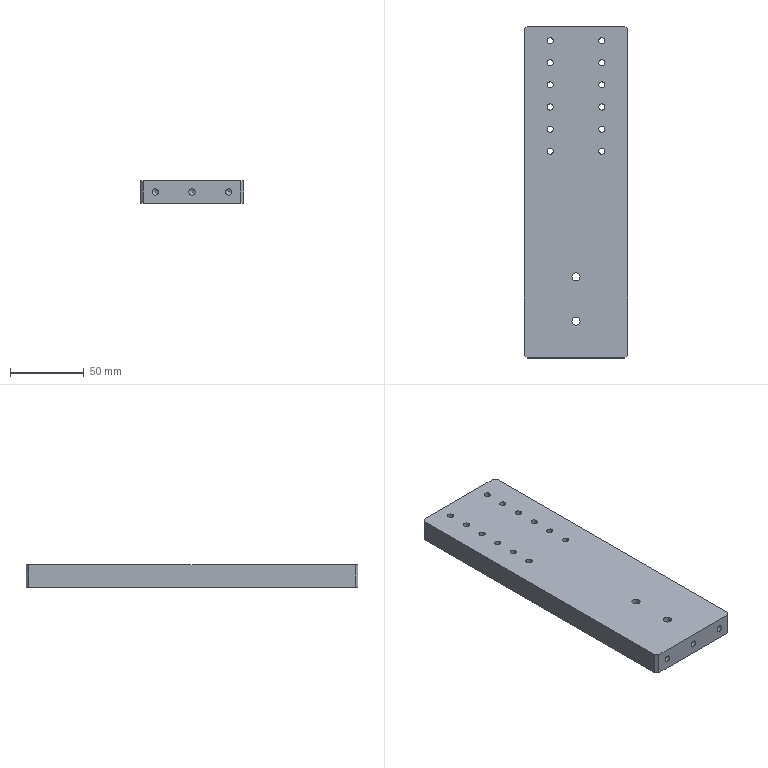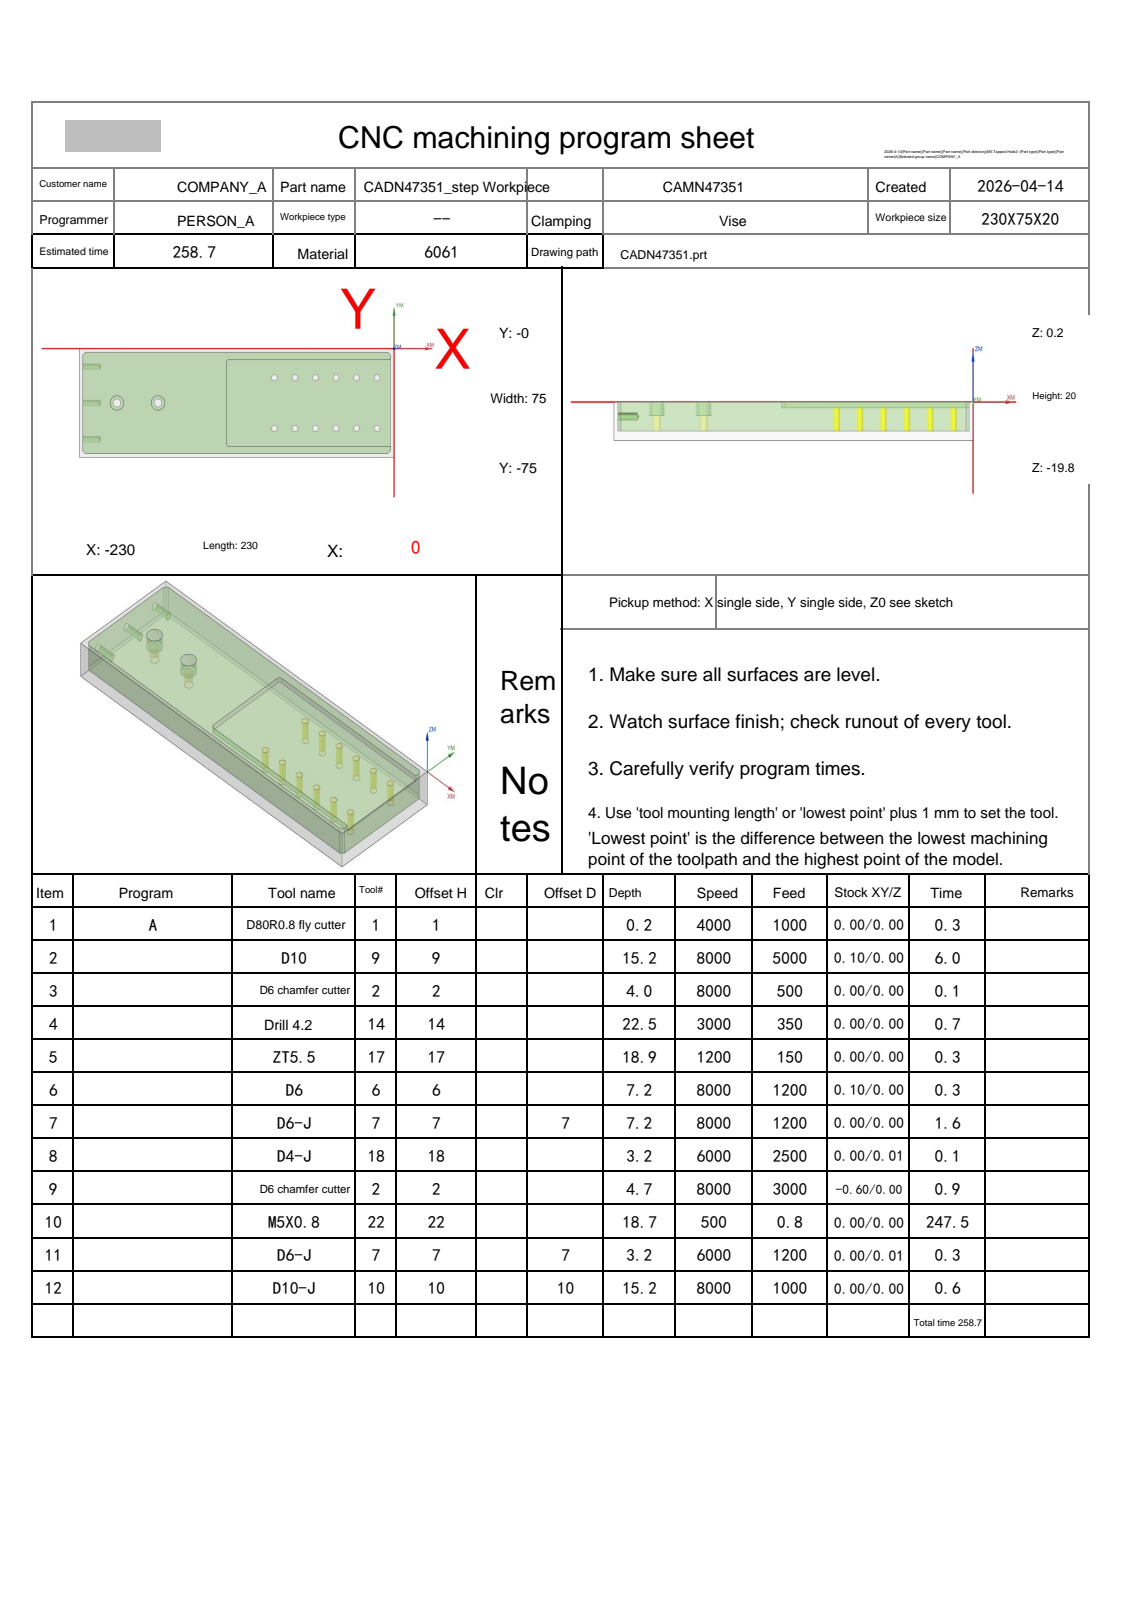NC program | NX | posted by the shop | part box 70 x 225 x 15 mm
Whole program, first 1531 of 2028 lines:
%
O0001
(Machine time: 493.75 MIN)
(===Total Tool:10===)
(T1=D80R0.8 fly cutter D=80.  R=0.8  D-  H01 Z=0.    )
(T9=D10     D=10.  R=0.   D-  H09 Z=-15.2 )
(T2=D6 chamfer cutter   D=6.   R=0.   D-  H02 Z=-4.5  )
(T14=Drill 4.2  D=4.2  DR_a=118 D-  H14 Z=-22.26)
(T17=ZT5.5  D=5.5  DR_a=118 D-  H17 Z=-18.65)
(T6=D6      D=6.   R=0.   D-  H06 Z=-7.   )
(T7=D6-J    D=6.   R=0.   D7  H07 Z=-7.   )
(T18=D4-J   D=4.   R=0.   D-  H18 Z=-3.   )
(T22=M5X0.8 D=4.2  DR_a=180 D-  H22 Z=-18.5 )
(T10=D10-J  D=10.  R=0.   D10 H10 Z=-15.2 )
G80 G90 G17 G49 G40
G91 G28 Z0
M01
N1 T01 M06
(D80R0.8 fly cutter  D=80. R=0.8 H=01 ce=0.00 di=0.00)
G00 G90 G54 X-272.5 Y-37.5 M03 S4000
G43 H01 Z20.
M08
Z2.
G01 Z0.0 F1000.
X-267.5
X37.5
X42.5
Z2.
G00 Z20.
G91 G28 Z0.0
M05
M09
G91 G28 Z0.0
M01
N2 T09 M06
(D10  D=10. R=0. H=09 ce=0.10 di=0.00)
G00 G90 G54 X-115. Y2.6 M03 S8000
G43 H09 Z20.
M08
Z.5
G01 X-4.5 Z.412 F5000.
G02 X-.894 Y1.106 Z.409 I0.0 J-5.1
G01 X1.106 Y-.894 Z.407
G02 X2.6 Y-4.5 Z.404 I-3.606 J-3.606
G01 Y-70.5 Z.351
G02 X1.106 Y-74.106 Z.348 I-5.1 J0.0
G01 X-.894 Y-76.106 Z.346
G02 X-4.5 Y-77.6 Z.343 I-3.606 J3.606
G01 X-225.5 Z.167
G02 X-229.106 Y-76.106 Z.164 I0.0 J5.1
G01 X-231.106 Y-74.106 Z.161
G02 X-232.6 Y-70.5 Z.158 I3.606 J3.606
G01 Y-4.5 Z.106
G02 X-231.106 Y-.894 Z.103 I5.1 J0.0
G01 X-229.106 Y1.106 Z.1
G02 X-225.5 Y2.6 Z.097 I3.606 J-3.606
G01 X-4.5 Z-.078
G02 X-.894 Y1.106 Z-.082 I0.0 J-5.1
G01 X1.106 Y-.894 Z-.084
G02 X2.6 Y-4.5 Z-.087 I-3.606 J-3.606
G01 Y-70.5 Z-.14
G02 X1.106 Y-74.106 Z-.143 I-5.1 J0.0
G01 X-.894 Y-76.106 Z-.145
G02 X-4.5 Y-77.6 Z-.148 I-3.606 J3.606
G01 X-225.5 Z-.324
G02 X-229.106 Y-76.106 Z-.327 I0.0 J5.1
G01 X-231.106 Y-74.106 Z-.329
G02 X-232.6 Y-70.5 Z-.332 I3.606 J3.606
G01 Y-4.5 Z-.385
G02 X-231.106 Y-.894 Z-.388 I5.1 J0.0
G01 X-229.106 Y1.106 Z-.39
G02 X-225.5 Y2.6 Z-.393 I3.606 J-3.606
G01 X-4.5 Z-.569
G02 X-.894 Y1.106 Z-.572 I0.0 J-5.1
G01 X1.106 Y-.894 Z-.574
G02 X2.6 Y-4.5 Z-.578 I-3.606 J-3.606
G01 Y-70.5 Z-.63
G02 X1.106 Y-74.106 Z-.633 I-5.1 J0.0
G01 X-.894 Y-76.106 Z-.636
G02 X-4.5 Y-77.6 Z-.639 I-3.606 J3.606
G01 X-225.5 Z-.814
G02 X-229.106 Y-76.106 Z-.818 I0.0 J5.1
G01 X-231.106 Y-74.106 Z-.82
G02 X-232.6 Y-70.5 Z-.823 I3.606 J3.606
G01 Y-4.5 Z-.875
G02 X-231.106 Y-.894 Z-.879 I5.1 J0.0
G01 X-229.106 Y1.106 Z-.881
G02 X-225.5 Y2.6 Z-.884 I3.606 J-3.606
G01 X-4.5 Z-1.06
G02 X-.894 Y1.106 Z-1.063 I0.0 J-5.1
G01 X1.106 Y-.894 Z-1.065
G02 X2.6 Y-4.5 Z-1.068 I-3.606 J-3.606
G01 Y-70.5 Z-1.121
G02 X1.106 Y-74.106 Z-1.124 I-5.1 J0.0
G01 X-.894 Y-76.106 Z-1.126
G02 X-4.5 Y-77.6 Z-1.129 I-3.606 J3.606
G01 X-225.5 Z-1.305
G02 X-229.106 Y-76.106 Z-1.308 I0.0 J5.1
G01 X-231.106 Y-74.106 Z-1.31
G02 X-232.6 Y-70.5 Z-1.314 I3.606 J3.606
G01 Y-4.5 Z-1.366
G02 X-231.106 Y-.894 Z-1.369 I5.1 J0.0
G01 X-229.106 Y1.106 Z-1.372
G02 X-225.5 Y2.6 Z-1.375 I3.606 J-3.606
G01 X-4.5 Z-1.55
G02 X-.894 Y1.106 Z-1.554 I0.0 J-5.1
G01 X1.106 Y-.894 Z-1.556
G02 X2.6 Y-4.5 Z-1.559 I-3.606 J-3.606
G01 Y-70.5 Z-1.611
G02 X1.106 Y-74.106 Z-1.615 I-5.1 J0.0
G01 X-.894 Y-76.106 Z-1.617
G02 X-4.5 Y-77.6 Z-1.62 I-3.606 J3.606
G01 X-225.5 Z-1.796
G02 X-229.106 Y-76.106 Z-1.799 I0.0 J5.1
G01 X-231.106 Y-74.106 Z-1.801
G02 X-232.6 Y-70.5 Z-1.804 I3.606 J3.606
G01 Y-4.5 Z-1.857
G02 X-231.106 Y-.894 Z-1.86 I5.1 J0.0
G01 X-229.106 Y1.106 Z-1.862
G02 X-225.5 Y2.6 Z-1.865 I3.606 J-3.606
G01 X-4.5 Z-2.041
G02 X-.894 Y1.106 Z-2.044 I0.0 J-5.1
G01 X1.106 Y-.894 Z-2.046
G02 X2.6 Y-4.5 Z-2.05 I-3.606 J-3.606
G01 Y-70.5 Z-2.102
G02 X1.106 Y-74.106 Z-2.105 I-5.1 J0.0
G01 X-.894 Y-76.106 Z-2.107
G02 X-4.5 Y-77.6 Z-2.111 I-3.606 J3.606
G01 X-225.5 Z-2.286
G02 X-229.106 Y-76.106 Z-2.289 I0.0 J5.1
G01 X-231.106 Y-74.106 Z-2.292
G02 X-232.6 Y-70.5 Z-2.295 I3.606 J3.606
G01 Y-4.5 Z-2.347
G02 X-231.106 Y-.894 Z-2.351 I5.1 J0.0
G01 X-229.106 Y1.106 Z-2.353
G02 X-225.5 Y2.6 Z-2.356 I3.606 J-3.606
G01 X-4.5 Z-2.532
G02 X-.894 Y1.106 Z-2.535 I0.0 J-5.1
G01 X1.106 Y-.894 Z-2.537
G02 X2.6 Y-4.5 Z-2.54 I-3.606 J-3.606
G01 Y-70.5 Z-2.593
G02 X1.106 Y-74.106 Z-2.596 I-5.1 J0.0
G01 X-.894 Y-76.106 Z-2.598
G02 X-4.5 Y-77.6 Z-2.601 I-3.606 J3.606
G01 X-225.5 Z-2.777
G02 X-229.106 Y-76.106 Z-2.78 I0.0 J5.1
G01 X-231.106 Y-74.106 Z-2.782
G02 X-232.6 Y-70.5 Z-2.785 I3.606 J3.606
G01 Y-4.5 Z-2.838
G02 X-231.106 Y-.894 Z-2.841 I5.1 J0.0
G01 X-229.106 Y1.106 Z-2.843
G02 X-225.5 Y2.6 Z-2.847 I3.606 J-3.606
G01 X-4.5 Z-3.022
G02 X-.894 Y1.106 Z-3.025 I0.0 J-5.1
G01 X1.106 Y-.894 Z-3.028
G02 X2.6 Y-4.5 Z-3.031 I-3.606 J-3.606
G01 Y-70.5 Z-3.083
G02 X1.106 Y-74.106 Z-3.086 I-5.1 J0.0
G01 X-.894 Y-76.106 Z-3.089
G02 X-4.5 Y-77.6 Z-3.092 I-3.606 J3.606
G01 X-225.5 Z-3.268
G02 X-229.106 Y-76.106 Z-3.271 I0.0 J5.1
G01 X-231.106 Y-74.106 Z-3.273
G02 X-232.6 Y-70.5 Z-3.276 I3.606 J3.606
G01 Y-4.5 Z-3.329
G02 X-231.106 Y-.894 Z-3.332 I5.1 J0.0
G01 X-229.106 Y1.106 Z-3.334
G02 X-225.5 Y2.6 Z-3.337 I3.606 J-3.606
G01 X-4.5 Z-3.513
G02 X-.894 Y1.106 Z-3.516 I0.0 J-5.1
G01 X1.106 Y-.894 Z-3.518
G02 X2.6 Y-4.5 Z-3.521 I-3.606 J-3.606
G01 Y-70.5 Z-3.574
G02 X1.106 Y-74.106 Z-3.577 I-5.1 J0.0
G01 X-.894 Y-76.106 Z-3.579
G02 X-4.5 Y-77.6 Z-3.582 I-3.606 J3.606
G01 X-225.5 Z-3.758
G02 X-229.106 Y-76.106 Z-3.761 I0.0 J5.1
G01 X-231.106 Y-74.106 Z-3.764
G02 X-232.6 Y-70.5 Z-3.767 I3.606 J3.606
G01 Y-4.5 Z-3.819
G02 X-231.106 Y-.894 Z-3.822 I5.1 J0.0
G01 X-229.106 Y1.106 Z-3.825
G02 X-225.5 Y2.6 Z-3.828 I3.606 J-3.606
G01 X-4.5 Z-4.003
G02 X-.894 Y1.106 Z-4.007 I0.0 J-5.1
G01 X1.106 Y-.894 Z-4.009
G02 X2.6 Y-4.5 Z-4.012 I-3.606 J-3.606
G01 Y-70.5 Z-4.065
G02 X1.106 Y-74.106 Z-4.068 I-5.1 J0.0
G01 X-.894 Y-76.106 Z-4.07
G02 X-4.5 Y-77.6 Z-4.073 I-3.606 J3.606
G01 X-225.5 Z-4.249
G02 X-229.106 Y-76.106 Z-4.252 I0.0 J5.1
G01 X-231.106 Y-74.106 Z-4.254
G02 X-232.6 Y-70.5 Z-4.257 I3.606 J3.606
G01 Y-4.5 Z-4.31
G02 X-231.106 Y-.894 Z-4.313 I5.1 J0.0
G01 X-229.106 Y1.106 Z-4.315
G02 X-225.5 Y2.6 Z-4.318 I3.606 J-3.606
G01 X-4.5 Z-4.494
G02 X-.894 Y1.106 Z-4.497 I0.0 J-5.1
G01 X1.106 Y-.894 Z-4.499
G02 X2.6 Y-4.5 Z-4.503 I-3.606 J-3.606
G01 Y-70.5 Z-4.555
G02 X1.106 Y-74.106 Z-4.558 I-5.1 J0.0
G01 X-.894 Y-76.106 Z-4.561
G02 X-4.5 Y-77.6 Z-4.564 I-3.606 J3.606
G01 X-225.5 Z-4.739
G02 X-229.106 Y-76.106 Z-4.743 I0.0 J5.1
G01 X-231.106 Y-74.106 Z-4.745
G02 X-232.6 Y-70.5 Z-4.748 I3.606 J3.606
G01 Y-4.5 Z-4.8
G02 X-231.106 Y-.894 Z-4.804 I5.1 J0.0
G01 X-229.106 Y1.106 Z-4.806
G02 X-225.5 Y2.6 Z-4.809 I3.606 J-3.606
G01 X-4.5 Z-4.985
G02 X-.894 Y1.106 Z-4.988 I0.0 J-5.1
G01 X1.106 Y-.894 Z-4.99
G02 X2.6 Y-4.5 Z-4.993 I-3.606 J-3.606
G01 Y-70.5 Z-5.046
G02 X1.106 Y-74.106 Z-5.049 I-5.1 J0.0
G01 X-.894 Y-76.106 Z-5.051
G02 X-4.5 Y-77.6 Z-5.054 I-3.606 J3.606
G01 X-225.5 Z-5.23
G02 X-229.106 Y-76.106 Z-5.233 I0.0 J5.1
G01 X-231.106 Y-74.106 Z-5.235
G02 X-232.6 Y-70.5 Z-5.239 I3.606 J3.606
G01 Y-4.5 Z-5.291
G02 X-231.106 Y-.894 Z-5.294 I5.1 J0.0
G01 X-229.106 Y1.106 Z-5.297
G02 X-225.5 Y2.6 Z-5.3 I3.606 J-3.606
G01 X-4.5 Z-5.475
G02 X-.894 Y1.106 Z-5.479 I0.0 J-5.1
G01 X1.106 Y-.894 Z-5.481
G02 X2.6 Y-4.5 Z-5.484 I-3.606 J-3.606
G01 Y-70.5 Z-5.536
G02 X1.106 Y-74.106 Z-5.54 I-5.1 J0.0
G01 X-.894 Y-76.106 Z-5.542
G02 X-4.5 Y-77.6 Z-5.545 I-3.606 J3.606
G01 X-225.5 Z-5.721
G02 X-229.106 Y-76.106 Z-5.724 I0.0 J5.1
G01 X-231.106 Y-74.106 Z-5.726
G02 X-232.6 Y-70.5 Z-5.729 I3.606 J3.606
G01 Y-4.5 Z-5.782
G02 X-231.106 Y-.894 Z-5.785 I5.1 J0.0
G01 X-229.106 Y1.106 Z-5.787
G02 X-225.5 Y2.6 Z-5.79 I3.606 J-3.606
G01 X-4.5 Z-5.966
G02 X-.894 Y1.106 Z-5.969 I0.0 J-5.1
G01 X1.106 Y-.894 Z-5.971
G02 X2.6 Y-4.5 Z-5.975 I-3.606 J-3.606
G01 Y-70.5 Z-6.027
G02 X1.106 Y-74.106 Z-6.03 I-5.1 J0.0
G01 X-.894 Y-76.106 Z-6.032
G02 X-4.5 Y-77.6 Z-6.036 I-3.606 J3.606
G01 X-225.5 Z-6.211
G02 X-229.106 Y-76.106 Z-6.214 I0.0 J5.1
G01 X-231.106 Y-74.106 Z-6.217
G02 X-232.6 Y-70.5 Z-6.22 I3.606 J3.606
G01 Y-4.5 Z-6.272
G02 X-231.106 Y-.894 Z-6.276 I5.1 J0.0
G01 X-229.106 Y1.106 Z-6.278
G02 X-225.5 Y2.6 Z-6.281 I3.606 J-3.606
G01 X-4.5 Z-6.457
G02 X-.894 Y1.106 Z-6.46 I0.0 J-5.1
G01 X1.106 Y-.894 Z-6.462
G02 X2.6 Y-4.5 Z-6.465 I-3.606 J-3.606
G01 Y-70.5 Z-6.518
G02 X1.106 Y-74.106 Z-6.521 I-5.1 J0.0
G01 X-.894 Y-76.106 Z-6.523
G02 X-4.5 Y-77.6 Z-6.526 I-3.606 J3.606
G01 X-225.5 Z-6.702
G02 X-229.106 Y-76.106 Z-6.705 I0.0 J5.1
G01 X-231.106 Y-74.106 Z-6.707
G02 X-232.6 Y-70.5 Z-6.71 I3.606 J3.606
G01 Y-4.5 Z-6.763
G02 X-231.106 Y-.894 Z-6.766 I5.1 J0.0
G01 X-229.106 Y1.106 Z-6.768
G02 X-225.5 Y2.6 Z-6.772 I3.606 J-3.606
G01 X-4.5 Z-6.947
G02 X-.894 Y1.106 Z-6.95 I0.0 J-5.1
G01 X1.106 Y-.894 Z-6.953
G02 X2.6 Y-4.5 Z-6.956 I-3.606 J-3.606
G01 Y-70.5 Z-7.008
G02 X1.106 Y-74.106 Z-7.011 I-5.1 J0.0
G01 X-.894 Y-76.106 Z-7.014
G02 X-4.5 Y-77.6 Z-7.017 I-3.606 J3.606
G01 X-225.5 Z-7.193
G02 X-229.106 Y-76.106 Z-7.196 I0.0 J5.1
G01 X-231.106 Y-74.106 Z-7.198
G02 X-232.6 Y-70.5 Z-7.201 I3.606 J3.606
G01 Y-4.5 Z-7.254
G02 X-231.106 Y-.894 Z-7.257 I5.1 J0.0
G01 X-229.106 Y1.106 Z-7.259
G02 X-225.5 Y2.6 Z-7.262 I3.606 J-3.606
G01 X-4.5 Z-7.438
G02 X-.894 Y1.106 Z-7.441 I0.0 J-5.1
G01 X1.106 Y-.894 Z-7.443
G02 X2.6 Y-4.5 Z-7.446 I-3.606 J-3.606
G01 Y-70.5 Z-7.499
G02 X1.106 Y-74.106 Z-7.502 I-5.1 J0.0
G01 X-.894 Y-76.106 Z-7.504
G02 X-4.5 Y-77.6 Z-7.507 I-3.606 J3.606
G01 X-225.5 Z-7.683
G02 X-229.106 Y-76.106 Z-7.686 I0.0 J5.1
G01 X-231.106 Y-74.106 Z-7.689
G02 X-232.6 Y-70.5 Z-7.692 I3.606 J3.606
G01 Y-4.5 Z-7.744
G02 X-231.106 Y-.894 Z-7.747 I5.1 J0.0
G01 X-229.106 Y1.106 Z-7.75
G02 X-225.5 Y2.6 Z-7.753 I3.606 J-3.606
G01 X-4.5 Z-7.928
G02 X-.894 Y1.106 Z-7.932 I0.0 J-5.1
G01 X1.106 Y-.894 Z-7.934
G02 X2.6 Y-4.5 Z-7.937 I-3.606 J-3.606
G01 Y-70.5 Z-7.99
G02 X1.106 Y-74.106 Z-7.993 I-5.1 J0.0
G01 X-.894 Y-76.106 Z-7.995
G02 X-4.5 Y-77.6 Z-7.998 I-3.606 J3.606
G01 X-225.5 Z-8.174
G02 X-229.106 Y-76.106 Z-8.177 I0.0 J5.1
G01 X-231.106 Y-74.106 Z-8.179
G02 X-232.6 Y-70.5 Z-8.182 I3.606 J3.606
G01 Y-4.5 Z-8.235
G02 X-231.106 Y-.894 Z-8.238 I5.1 J0.0
G01 X-229.106 Y1.106 Z-8.24
G02 X-225.5 Y2.6 Z-8.243 I3.606 J-3.606
G01 X-4.5 Z-8.419
G02 X-.894 Y1.106 Z-8.422 I0.0 J-5.1
G01 X1.106 Y-.894 Z-8.424
G02 X2.6 Y-4.5 Z-8.428 I-3.606 J-3.606
G01 Y-70.5 Z-8.48
G02 X1.106 Y-74.106 Z-8.483 I-5.1 J0.0
G01 X-.894 Y-76.106 Z-8.486
G02 X-4.5 Y-77.6 Z-8.489 I-3.606 J3.606
G01 X-225.5 Z-8.664
G02 X-229.106 Y-76.106 Z-8.668 I0.0 J5.1
G01 X-231.106 Y-74.106 Z-8.67
G02 X-232.6 Y-70.5 Z-8.673 I3.606 J3.606
G01 Y-4.5 Z-8.725
G02 X-231.106 Y-.894 Z-8.729 I5.1 J0.0
G01 X-229.106 Y1.106 Z-8.731
G02 X-225.5 Y2.6 Z-8.734 I3.606 J-3.606
G01 X-4.5 Z-8.91
G02 X-.894 Y1.106 Z-8.913 I0.0 J-5.1
G01 X1.106 Y-.894 Z-8.915
G02 X2.6 Y-4.5 Z-8.918 I-3.606 J-3.606
G01 Y-70.5 Z-8.971
G02 X1.106 Y-74.106 Z-8.974 I-5.1 J0.0
G01 X-.894 Y-76.106 Z-8.976
G02 X-4.5 Y-77.6 Z-8.979 I-3.606 J3.606
G01 X-225.5 Z-9.155
G02 X-229.106 Y-76.106 Z-9.158 I0.0 J5.1
G01 X-231.106 Y-74.106 Z-9.16
G02 X-232.6 Y-70.5 Z-9.164 I3.606 J3.606
G01 Y-4.5 Z-9.216
G02 X-231.106 Y-.894 Z-9.219 I5.1 J0.0
G01 X-229.106 Y1.106 Z-9.222
G02 X-225.5 Y2.6 Z-9.225 I3.606 J-3.606
G01 X-4.5 Z-9.4
G02 X-.894 Y1.106 Z-9.404 I0.0 J-5.1
G01 X1.106 Y-.894 Z-9.406
G02 X2.6 Y-4.5 Z-9.409 I-3.606 J-3.606
G01 Y-70.5 Z-9.461
G02 X1.106 Y-74.106 Z-9.465 I-5.1 J0.0
G01 X-.894 Y-76.106 Z-9.467
G02 X-4.5 Y-77.6 Z-9.47 I-3.606 J3.606
G01 X-225.5 Z-9.646
G02 X-229.106 Y-76.106 Z-9.649 I0.0 J5.1
G01 X-231.106 Y-74.106 Z-9.651
G02 X-232.6 Y-70.5 Z-9.654 I3.606 J3.606
G01 Y-4.5 Z-9.707
G02 X-231.106 Y-.894 Z-9.71 I5.1 J0.0
G01 X-229.106 Y1.106 Z-9.712
G02 X-225.5 Y2.6 Z-9.715 I3.606 J-3.606
G01 X-4.5 Z-9.891
G02 X-.894 Y1.106 Z-9.894 I0.0 J-5.1
G01 X1.106 Y-.894 Z-9.896
G02 X2.6 Y-4.5 Z-9.9 I-3.606 J-3.606
G01 Y-70.5 Z-9.952
G02 X1.106 Y-74.106 Z-9.955 I-5.1 J0.0
G01 X-.894 Y-76.106 Z-9.957
G02 X-4.5 Y-77.6 Z-9.961 I-3.606 J3.606
G01 X-225.5 Z-10.136
G02 X-229.106 Y-76.106 Z-10.139 I0.0 J5.1
G01 X-231.106 Y-74.106 Z-10.142
G02 X-232.6 Y-70.5 Z-10.145 I3.606 J3.606
G01 Y-4.5 Z-10.197
G02 X-231.106 Y-.894 Z-10.201 I5.1 J0.0
G01 X-229.106 Y1.106 Z-10.203
G02 X-225.5 Y2.6 Z-10.206 I3.606 J-3.606
G01 X-4.5 Z-10.382
G02 X-.894 Y1.106 Z-10.385 I0.0 J-5.1
G01 X1.106 Y-.894 Z-10.387
G02 X2.6 Y-4.5 Z-10.39 I-3.606 J-3.606
G01 Y-70.5 Z-10.443
G02 X1.106 Y-74.106 Z-10.446 I-5.1 J0.0
G01 X-.894 Y-76.106 Z-10.448
G02 X-4.5 Y-77.6 Z-10.451 I-3.606 J3.606
G01 X-225.5 Z-10.627
G02 X-229.106 Y-76.106 Z-10.63 I0.0 J5.1
G01 X-231.106 Y-74.106 Z-10.632
G02 X-232.6 Y-70.5 Z-10.635 I3.606 J3.606
G01 Y-4.5 Z-10.688
G02 X-231.106 Y-.894 Z-10.691 I5.1 J0.0
G01 X-229.106 Y1.106 Z-10.693
G02 X-225.5 Y2.6 Z-10.697 I3.606 J-3.606
G01 X-4.5 Z-10.872
G02 X-.894 Y1.106 Z-10.875 I0.0 J-5.1
G01 X1.106 Y-.894 Z-10.878
G02 X2.6 Y-4.5 Z-10.881 I-3.606 J-3.606
G01 Y-70.5 Z-10.933
G02 X1.106 Y-74.106 Z-10.936 I-5.1 J0.0
G01 X-.894 Y-76.106 Z-10.939
G02 X-4.5 Y-77.6 Z-10.942 I-3.606 J3.606
G01 X-225.5 Z-11.118
G02 X-229.106 Y-76.106 Z-11.121 I0.0 J5.1
G01 X-231.106 Y-74.106 Z-11.123
G02 X-232.6 Y-70.5 Z-11.126 I3.606 J3.606
G01 Y-4.5 Z-11.179
G02 X-231.106 Y-.894 Z-11.182 I5.1 J0.0
G01 X-229.106 Y1.106 Z-11.184
G02 X-225.5 Y2.6 Z-11.187 I3.606 J-3.606
G01 X-4.5 Z-11.363
G02 X-.894 Y1.106 Z-11.366 I0.0 J-5.1
G01 X1.106 Y-.894 Z-11.368
G02 X2.6 Y-4.5 Z-11.371 I-3.606 J-3.606
G01 Y-70.5 Z-11.424
G02 X1.106 Y-74.106 Z-11.427 I-5.1 J0.0
G01 X-.894 Y-76.106 Z-11.429
G02 X-4.5 Y-77.6 Z-11.432 I-3.606 J3.606
G01 X-225.5 Z-11.608
G02 X-229.106 Y-76.106 Z-11.611 I0.0 J5.1
G01 X-231.106 Y-74.106 Z-11.614
G02 X-232.6 Y-70.5 Z-11.617 I3.606 J3.606
G01 Y-4.5 Z-11.669
G02 X-231.106 Y-.894 Z-11.672 I5.1 J0.0
G01 X-229.106 Y1.106 Z-11.675
G02 X-225.5 Y2.6 Z-11.678 I3.606 J-3.606
G01 X-4.5 Z-11.853
G02 X-.894 Y1.106 Z-11.857 I0.0 J-5.1
G01 X1.106 Y-.894 Z-11.859
G02 X2.6 Y-4.5 Z-11.862 I-3.606 J-3.606
G01 Y-70.5 Z-11.915
G02 X1.106 Y-74.106 Z-11.918 I-5.1 J0.0
G01 X-.894 Y-76.106 Z-11.92
G02 X-4.5 Y-77.6 Z-11.923 I-3.606 J3.606
G01 X-225.5 Z-12.099
G02 X-229.106 Y-76.106 Z-12.102 I0.0 J5.1
G01 X-231.106 Y-74.106 Z-12.104
G02 X-232.6 Y-70.5 Z-12.107 I3.606 J3.606
G01 Y-4.5 Z-12.16
G02 X-231.106 Y-.894 Z-12.163 I5.1 J0.0
G01 X-229.106 Y1.106 Z-12.165
G02 X-225.5 Y2.6 Z-12.168 I3.606 J-3.606
G01 X-4.5 Z-12.344
G02 X-.894 Y1.106 Z-12.347 I0.0 J-5.1
G01 X1.106 Y-.894 Z-12.349
G02 X2.6 Y-4.5 Z-12.353 I-3.606 J-3.606
G01 Y-70.5 Z-12.405
G02 X1.106 Y-74.106 Z-12.408 I-5.1 J0.0
G01 X-.894 Y-76.106 Z-12.411
G02 X-4.5 Y-77.6 Z-12.414 I-3.606 J3.606
G01 X-225.5 Z-12.589
G02 X-229.106 Y-76.106 Z-12.593 I0.0 J5.1
G01 X-231.106 Y-74.106 Z-12.595
G02 X-232.6 Y-70.5 Z-12.598 I3.606 J3.606
G01 Y-4.5 Z-12.65
G02 X-231.106 Y-.894 Z-12.654 I5.1 J0.0
G01 X-229.106 Y1.106 Z-12.656
G02 X-225.5 Y2.6 Z-12.659 I3.606 J-3.606
G01 X-4.5 Z-12.835
G02 X-.894 Y1.106 Z-12.838 I0.0 J-5.1
G01 X1.106 Y-.894 Z-12.84
G02 X2.6 Y-4.5 Z-12.843 I-3.606 J-3.606
G01 Y-70.5 Z-12.896
G02 X1.106 Y-74.106 Z-12.899 I-5.1 J0.0
G01 X-.894 Y-76.106 Z-12.901
G02 X-4.5 Y-77.6 Z-12.904 I-3.606 J3.606
G01 X-225.5 Z-13.08
G02 X-229.106 Y-76.106 Z-13.083 I0.0 J5.1
G01 X-231.106 Y-74.106 Z-13.085
G02 X-232.6 Y-70.5 Z-13.089 I3.606 J3.606
G01 Y-4.5 Z-13.141
G02 X-231.106 Y-.894 Z-13.144 I5.1 J0.0
G01 X-229.106 Y1.106 Z-13.147
G02 X-225.5 Y2.6 Z-13.15 I3.606 J-3.606
G01 X-4.5 Z-13.325
G02 X-.894 Y1.106 Z-13.329 I0.0 J-5.1
G01 X1.106 Y-.894 Z-13.331
G02 X2.6 Y-4.5 Z-13.334 I-3.606 J-3.606
G01 Y-70.5 Z-13.386
G02 X1.106 Y-74.106 Z-13.39 I-5.1 J0.0
G01 X-.894 Y-76.106 Z-13.392
G02 X-4.5 Y-77.6 Z-13.395 I-3.606 J3.606
G01 X-225.5 Z-13.571
G02 X-229.106 Y-76.106 Z-13.574 I0.0 J5.1
G01 X-231.106 Y-74.106 Z-13.576
G02 X-232.6 Y-70.5 Z-13.579 I3.606 J3.606
G01 Y-4.5 Z-13.632
G02 X-231.106 Y-.894 Z-13.635 I5.1 J0.0
G01 X-229.106 Y1.106 Z-13.637
G02 X-225.5 Y2.6 Z-13.64 I3.606 J-3.606
G01 X-4.5 Z-13.816
G02 X-.894 Y1.106 Z-13.819 I0.0 J-5.1
G01 X1.106 Y-.894 Z-13.821
G02 X2.6 Y-4.5 Z-13.825 I-3.606 J-3.606
G01 Y-70.5 Z-13.877
G02 X1.106 Y-74.106 Z-13.88 I-5.1 J0.0
G01 X-.894 Y-76.106 Z-13.882
G02 X-4.5 Y-77.6 Z-13.886 I-3.606 J3.606
G01 X-225.5 Z-14.061
G02 X-229.106 Y-76.106 Z-14.064 I0.0 J5.1
G01 X-231.106 Y-74.106 Z-14.067
G02 X-232.6 Y-70.5 Z-14.07 I3.606 J3.606
G01 Y-4.5 Z-14.122
G02 X-231.106 Y-.894 Z-14.126 I5.1 J0.0
G01 X-229.106 Y1.106 Z-14.128
G02 X-225.5 Y2.6 Z-14.131 I3.606 J-3.606
G01 X-4.5 Z-14.307
G02 X-.894 Y1.106 Z-14.31 I0.0 J-5.1
G01 X1.106 Y-.894 Z-14.312
G02 X2.6 Y-4.5 Z-14.315 I-3.606 J-3.606
G01 Y-70.5 Z-14.368
G02 X1.106 Y-74.106 Z-14.371 I-5.1 J0.0
G01 X-.894 Y-76.106 Z-14.373
G02 X-4.5 Y-77.6 Z-14.376 I-3.606 J3.606
G01 X-225.5 Z-14.552
G02 X-229.106 Y-76.106 Z-14.555 I0.0 J5.1
G01 X-231.106 Y-74.106 Z-14.557
G02 X-232.6 Y-70.5 Z-14.56 I3.606 J3.606
G01 Y-4.5 Z-14.613
G02 X-231.106 Y-.894 Z-14.616 I5.1 J0.0
G01 X-229.106 Y1.106 Z-14.618
G02 X-225.5 Y2.6 Z-14.622 I3.606 J-3.606
G01 X-4.5 Z-14.797
G02 X-.894 Y1.106 Z-14.8 I0.0 J-5.1
G01 X1.106 Y-.894 Z-14.803
G02 X2.6 Y-4.5 Z-14.806 I-3.606 J-3.606
G01 Y-70.5 Z-14.858
G02 X1.106 Y-74.106 Z-14.861 I-5.1 J0.0
G01 X-.894 Y-76.106 Z-14.864
G02 X-4.5 Y-77.6 Z-14.867 I-3.606 J3.606
G01 X-225.5 Z-15.043
G02 X-229.106 Y-76.106 Z-15.046 I0.0 J5.1
G01 X-231.106 Y-74.106 Z-15.048
G02 X-232.6 Y-70.5 Z-15.051 I3.606 J3.606
G01 Y-4.5 Z-15.104
G02 X-231.106 Y-.894 Z-15.107 I5.1 J0.0
G01 X-229.106 Y1.106 Z-15.109
G02 X-225.5 Y2.6 Z-15.112 I3.606 J-3.606
G01 X-115. Z-15.2
X-4.5
G02 X-.894 Y1.106 I0.0 J-5.1
G01 X1.106 Y-.894
G02 X2.6 Y-4.5 I-3.606 J-3.606
G01 Y-70.5
G02 X1.106 Y-74.106 I-5.1 J0.0
G01 X-.894 Y-76.106
G02 X-4.5 Y-77.6 I-3.606 J3.606
G01 X-225.5
G02 X-229.106 Y-76.106 I0.0 J5.1
G01 X-231.106 Y-74.106
G02 X-232.6 Y-70.5 I3.606 J3.606
G01 Y-4.5
G02 X-231.106 Y-.894 I5.1 J0.0
G01 X-229.106 Y1.106
G02 X-225.5 Y2.6 I3.606 J-3.606
G01 X-115.
X-114.5
Z-14.2
G00 Z20.
G00 G90 X.52 Y-37.5 M03 S6000
Z20.
Z.257
G01 Z-.243 F3500.
X-2.48
Y-62.009
Y-62.4
X-9.48
X-117.4
Y-12.6
X-2.48
Y-12.991
Y-37.5
X-9.48
Y-55.4
X-110.4
Y-19.6
X-9.48
Y-37.5
X-16.48
Y-48.4
X-103.4
Y-26.6
X-16.48
Y-37.5
X-23.48
Y-41.4
X-96.4
Y-33.6
X-23.48
Y-37.5
Z.757
G00 Z1.2
X.52
Z-.186
G01 Z-.686
X-2.48
Y-62.009
Y-62.4
X-9.48
X-117.4
Y-12.6
X-2.48
Y-12.991
Y-37.5
X-9.48
Y-55.4
X-110.4
Y-19.6
X-9.48
Y-37.5
X-16.48
Y-48.4
X-103.4
Y-26.6
X-16.48
Y-37.5
X-23.48
Y-41.4
X-96.4
Y-33.6
X-23.48
Y-37.5
Z.314
G00 Z.757
X.52
Z-.629
G01 Z-1.129
X-2.48
Y-62.009
Y-62.4
X-9.48
X-117.4
Y-12.6
X-2.48
Y-12.991
Y-37.5
X-9.48
Y-55.4
X-110.4
Y-19.6
X-9.48
Y-37.5
X-16.48
Y-48.4
X-103.4
Y-26.6
X-16.48
Y-37.5
X-23.48
Y-41.4
X-96.4
Y-33.6
X-23.48
Y-37.5
Z-.129
G00 Z.314
X.52
Z-1.071
G01 Z-1.571
X-2.48
Y-62.009
Y-62.4
X-9.48
X-117.4
Y-12.6
X-2.48
Y-12.991
Y-37.5
X-9.48
Y-55.4
X-110.4
Y-19.6
X-9.48
Y-37.5
X-16.48
Y-48.4
X-103.4
Y-26.6
X-16.48
Y-37.5
X-23.48
Y-41.4
X-96.4
Y-33.6
X-23.48
Y-37.5
Z-.571
G00 Z-.129
X.52
Z-1.514
G01 Z-2.014
X-2.48
Y-62.009
Y-62.4
X-9.48
X-117.4
Y-12.6
X-2.48
Y-12.991
Y-37.5
X-9.48
Y-55.4
X-110.4
Y-19.6
X-9.48
Y-37.5
X-16.48
Y-48.4
X-103.4
Y-26.6
X-16.48
Y-37.5
X-23.48
Y-41.4
X-96.4
Y-33.6
X-23.48
Y-37.5
Z-1.014
G00 Z-.571
X.52
Z-1.957
G01 Z-2.457
X-2.48
Y-62.009
Y-62.4
X-9.48
X-117.4
Y-12.6
X-2.48
Y-12.991
Y-37.5
X-9.48
Y-55.4
X-110.4
Y-19.6
X-9.48
Y-37.5
X-16.48
Y-48.4
X-103.4
Y-26.6
X-16.48
Y-37.5
X-23.48
Y-41.4
X-96.4
Y-33.6
X-23.48
Y-37.5
Z-1.457
G00 Z-1.014
X.52
Z-2.4
G01 Z-2.9
X-2.48
Y-62.009
Y-62.4
X-9.48
X-117.4
Y-12.6
X-2.48
Y-12.991
Y-37.5
X-9.48
Y-55.4
X-110.4
Y-19.6
X-9.48
Y-37.5
X-16.48
Y-48.4
X-103.4
Y-26.6
X-16.48
Y-37.5
X-23.48
Y-41.4
X-96.4
Y-33.6
X-23.48
Y-37.5
Z-1.9
G00 Z20.
G91 G28 Z0.0
M05
M09
G91 G28 Z0.0
M01
N3 T02 M06
(D6 chamfer cutter  D=6. R=0. H=02 ce=0.00 di=0.10)
G00 G90 G54 X-87.429 Y-20. M03 S8000
G43 H02 Z20.
M08
G98 G81 X-87.429 Y-20. Z-3.8 R-2. F500.
X-72.429
X-57.429
X-42.429
X-27.429
X-12.429
Y-55.
X-27.429
X-42.429
X-57.429
X-72.429
X-87.429
X-172.5 Y-37.5 Z-.8 R1.
X-202.5
G80
G00 Z20.
G91 G28 Z0.0
M05
M09
G91 G28 Z0.0
M01
N4 T14 M06
(Drill 4.2 D=4.2 DR_a=118 H=14)
G00 G90 G54 X-87.429 Y-55. M03 S3000
G43 H14 Z20.
M08
G98 G83 X-87.429 Y-55. Z-22.262 R-2. F350. Q3.
X-72.429
X-57.429
X-42.429
X-27.429
X-12.429
Y-20.
X-27.429
X-42.429
X-57.429
X-72.429
X-87.429
G80
G00 Z20.
G91 G28 Z0.0
M05
M09
G91 G28 Z0.0
M01
N5 T17 M06
(ZT5.5 D=5.5 DR_a=118 H=17)
G00 G90 G54 X-202.5 Y-37.5 M03 S1200
G43 H17 Z20.
M08
G98 G83 X-202.5 Y-37.5 Z-18.652 R1. F150. Q2.
X-172.5
G80
G00 Z20.
G91 G28 Z0.0
M05
M09
G91 G28 Z0.0
M01
N6 T06 M06
(D6  D=6. R=0. H=06 ce=0.10 di=0.00)
G00 G90 G54 X-202.5 Y-37.5 M03 S8000
G43 H06 Z20.
M08
Z.5
G03 X-201.55 Y-36.55 I0.0 J.95 F1200.
X-202.5 Y-35.6 I-.95 J0.0
X-202.5 Y-35.6 Z0.0 I0.0 J-1.9
X-202.5 Y-35.6 Z-.5 I0.0 J-1.9
X-202.5 Y-35.6 Z-1. I0.0 J-1.9
X-202.5 Y-35.6 Z-1.5 I0.0 J-1.9
X-202.5 Y-35.6 Z-2. I0.0 J-1.9
X-202.5 Y-35.6 Z-2.5 I0.0 J-1.9
X-202.5 Y-35.6 Z-3. I0.0 J-1.9
X-202.5 Y-35.6 Z-3.5 I0.0 J-1.9
X-202.5 Y-35.6 Z-4. I0.0 J-1.9
X-202.5 Y-35.6 Z-4.5 I0.0 J-1.9
X-202.5 Y-35.6 Z-5. I0.0 J-1.9
X-202.5 Y-35.6 Z-5.5 I0.0 J-1.9
X-202.5 Y-35.6 Z-6. I0.0 J-1.9
X-202.5 Y-35.6 Z-6.5 I0.0 J-1.9
X-202.5 Y-35.6 Z-7. I0.0 J-1.9
X-204.4 Y-37.5 I0.0 J-1.9
X-202.5 Y-39.4 I1.9 J0.0
X-200.6 Y-37.5 I0.0 J1.9
X-202.5 Y-35.6 I-1.9 J0.0
X-203.45 Y-36.55 I0.0 J-.95
X-202.5 Y-37.5 I.95 J0.0
G00 Z20.
X-172.5
Z.5
G03 X-171.55 Y-36.55 I0.0 J.95
X-172.5 Y-35.6 I-.95 J0.0
X-172.5 Y-35.6 Z0.0 I0.0 J-1.9
X-172.5 Y-35.6 Z-.5 I0.0 J-1.9
X-172.5 Y-35.6 Z-1. I0.0 J-1.9
X-172.5 Y-35.6 Z-1.5 I0.0 J-1.9
X-172.5 Y-35.6 Z-2. I0.0 J-1.9
X-172.5 Y-35.6 Z-2.5 I0.0 J-1.9
X-172.5 Y-35.6 Z-3. I0.0 J-1.9
X-172.5 Y-35.6 Z-3.5 I0.0 J-1.9
X-172.5 Y-35.6 Z-4. I0.0 J-1.9
X-172.5 Y-35.6 Z-4.5 I0.0 J-1.9
X-172.5 Y-35.6 Z-5. I0.0 J-1.9
X-172.5 Y-35.6 Z-5.5 I0.0 J-1.9
X-172.5 Y-35.6 Z-6. I0.0 J-1.9
X-172.5 Y-35.6 Z-6.5 I0.0 J-1.9
X-172.5 Y-35.6 Z-7. I0.0 J-1.9
X-174.4 Y-37.5 I0.0 J-1.9
X-172.5 Y-39.4 I1.9 J0.0
X-170.6 Y-37.5 I0.0 J1.9
X-172.5 Y-35.6 I-1.9 J0.0
X-173.45 Y-36.55 I0.0 J-.95
X-172.5 Y-37.5 I.95 J0.0
G00 Z20.
G91 G28 Z0.0
M05
M09
G91 G28 Z0.0
M01
N7 T07 M06
(D6-J  D=6. R=0. H=07 ce=0.00 di=0.00)
G00 G90 G54 X-202.5 Y-37.5 M03 S8000
G43 H07 Z20.
M08
Z0.0
G41 D07
G01 X-202.304 Y-37.46 F1000.
G03 X-201.51 Y-36.49 I-.196 J.97
X-202.5 Y-35.5 I-.99 J0.0
X-202.5 Y-35.5 Z-5. I0.0 J-2.
X-203.676 Y-39.118 Z-7. I0.0 J-2.
X-202.5 Y-39.5 I1.176 J1.618
X-200.5 Y-37.5 I0.0 J2.
X-202.5 Y-35.5 I-2. J0.0
X-204.5 Y-37.5 I0.0 J-2.
X-203.676 Y-39.118 I2. J0.0
X-203.094 Y-39.307 I.582 J.801
X-202.104 Y-38.317 I0.0 J.99
X-202.365 Y-37.647 I-.99 J0.0
G01 G40 X-202.5 Y-37.5
G00 Z20.
X-172.5
Z0.0
G41 D07
G01 X-172.304 Y-37.46
G03 X-171.51 Y-36.49 I-.196 J.97
X-172.5 Y-35.5 I-.99 J0.0
X-172.5 Y-35.5 Z-5. I0.0 J-2.
X-173.676 Y-39.118 Z-7. I0.0 J-2.
X-172.5 Y-39.5 I1.176 J1.618
X-170.5 Y-37.5 I0.0 J2.
X-172.5 Y-35.5 I-2. J0.0
X-174.5 Y-37.5 I0.0 J-2.
X-173.676 Y-39.118 I2. J0.0
X-173.094 Y-39.307 I.582 J.801
X-172.104 Y-38.317 I0.0 J.99
X-172.365 Y-37.647 I-.99 J0.0
G01 G40 X-172.5 Y-37.5
G00 Z20.
G00 G90 X3.5 Y-37.5 M03 S6000
Z20.
Z-2.5
G01 Z-3. F1200.
X-1.9
Y-64.2
X-119.2
Y-10.8
X-1.9
Y-37.5
X-6.1
Y-60.
X-115.
Y-15.
X-6.1
Y-37.5
X-10.3
Y-55.8
X-110.8
Y-19.2
X-10.3
Y-37.5
X-14.5
Y-51.6
X-106.6
Y-23.4
X-14.5
Y-37.5
X-18.7
Y-47.4
X-102.4
Y-27.6
X-18.7
Y-37.5
X-22.9
Y-43.2
X-98.2
Y-31.8
X-22.9
Y-37.5
X-27.1
Y-39.
X-94.
Y-36.
X-27.1
Y-37.5
Y-38.
X-23.5
Z-2.5
G00 Z20.
G91 G28 Z0.0
M05
M09
G91 G28 Z0.0
M01
N8 T18 M06
(D4-J  D=4. R=0. H=18 ce=0.00 di=0.01)
G00 G90 G54 X-116.947 Y-10.1 M03 S6000
G43 H18 Z20.
M08
Z.301
G01 X-116.948 Y-10.093 Z.215 F2000.
X-116.951 Y-10.074 Z.137
X-116.956 Y-10.045 Z.067
X-116.964 Y-10.006 Z.004
X-116.975 Y-9.961 Z-.051
X-116.989 Y-9.91 Z-.1
X-117.006 Y-9.856 Z-.143
X-117.027 Y-9.8 Z-.18
X-117.051 Y-9.744 Z-.21
X-117.08 Y-9.69 Z-.236
X-117.112 Y-9.639 Z-.257
X-117.149 Y-9.594 Z-.273
X-117.191 Y-9.555 Z-.285
X-117.238 Y-9.526 Z-.293
X-117.29 Y-9.507 Z-.298
X-117.347 Y-9.5 Z-.3
X-120.487 F2500.
X-120.5
Y-12.653
X-120.484 Y-12.696
X-120.438 Y-12.718 Z-.303
X-120.366 Y-12.719 Z-.307
X-120.271 Y-12.702 Z-.313
X-120.156 Y-12.669 Z-.32
X-120.026 Y-12.62 Z-.328
X-119.882 Y-12.557 Z-.337
X-119.73 Y-12.483 Z-.347
X-119.571 Y-12.398 Z-.358
X-119.41 Y-12.304 Z-.369
X-119.25 Y-12.203 Z-.381
X-118.913 Y-11.962 Z-.407
X-118.597 Y-11.694 Z-.435
X-118.306 Y-11.403 Z-.463
X-118.038 Y-11.087 Z-.491
X-117.797 Y-10.75 Z-.518
X-117.696 Y-10.59 Z-.53
X-117.602 Y-10.429 Z-.541
X-117.517 Y-10.27 Z-.552
X-117.443 Y-10.118 Z-.562
X-117.38 Y-9.974 Z-.571
X-117.331 Y-9.844 Z-.579
X-117.298 Y-9.729 Z-.586
X-117.281 Y-9.634 Z-.591
X-117.282 Y-9.562 Z-.595
X-117.304 Y-9.516 Z-.598
X-117.347 Y-9.5 Z-.599
X-120.487
X-120.5
Y-12.653
X-120.484 Y-12.696 Z-.6
X-120.438 Y-12.718 Z-.603
X-120.366 Y-12.719 Z-.607
X-120.271 Y-12.702 Z-.612
X-120.156 Y-12.669 Z-.619
X-120.026 Y-12.62 Z-.627
X-119.882 Y-12.557 Z-.636
X-119.73 Y-12.483 Z-.646
X-119.571 Y-12.398 Z-.657
X-119.41 Y-12.304 Z-.668
X-119.25 Y-12.203 Z-.68
X-118.913 Y-11.962 Z-.707
X-118.597 Y-11.694 Z-.735
X-118.306 Y-11.403 Z-.763
X-118.038 Y-11.087 Z-.791
X-117.797 Y-10.75 Z-.817
X-117.696 Y-10.59 Z-.829
X-117.602 Y-10.429 Z-.84
X-117.517 Y-10.27 Z-.851
X-117.443 Y-10.118 Z-.861
X-117.38 Y-9.974 Z-.87
X-117.331 Y-9.844 Z-.878
X-117.298 Y-9.729 Z-.885
X-117.281 Y-9.634 Z-.891
X-117.282 Y-9.562 Z-.895
X-117.304 Y-9.516 Z-.898
X-117.347 Y-9.5 Z-.899
X-120.487
X-120.5
Y-12.653
X-120.484 Y-12.696
X-120.438 Y-12.718 Z-.902
X-120.366 Y-12.719 Z-.906
X-120.271 Y-12.702 Z-.912
X-120.156 Y-12.669 Z-.919
X-120.026 Y-12.62 Z-.927
X-119.882 Y-12.557 Z-.936
X-119.73 Y-12.483 Z-.946
X-119.571 Y-12.398 Z-.957
X-119.41 Y-12.304 Z-.968
X-119.25 Y-12.203 Z-.98
X-118.913 Y-11.962 Z-1.006
X-118.597 Y-11.694 Z-1.034
X-118.306 Y-11.403 Z-1.062
X-118.038 Y-11.087 Z-1.09
X-117.797 Y-10.75 Z-1.117
X-117.696 Y-10.59 Z-1.129
X-117.602 Y-10.429 Z-1.14
X-117.517 Y-10.27 Z-1.151
X-117.443 Y-10.118 Z-1.161
X-117.38 Y-9.974 Z-1.17
X-117.331 Y-9.844 Z-1.178
X-117.298 Y-9.729 Z-1.185
X-117.281 Y-9.634 Z-1.19
X-117.282 Y-9.562 Z-1.194
X-117.304 Y-9.516 Z-1.197
X-117.347 Y-9.5 Z-1.198
X-120.487
X-120.5
Y-12.653
X-120.484 Y-12.696 Z-1.199
X-120.438 Y-12.718 Z-1.202
X-120.366 Y-12.719 Z-1.206
X-120.271 Y-12.702 Z-1.211
X-120.156 Y-12.669 Z-1.218
X-120.026 Y-12.62 Z-1.226
X-119.882 Y-12.557 Z-1.235
X-119.73 Y-12.483 Z-1.245
X-119.571 Y-12.398 Z-1.256
X-119.41 Y-12.304 Z-1.267
X-119.25 Y-12.203 Z-1.279
X-118.913 Y-11.962 Z-1.306
X-118.597 Y-11.694 Z-1.334
X-118.306 Y-11.403 Z-1.362
X-118.038 Y-11.087 Z-1.39
X-117.797 Y-10.75 Z-1.416
X-117.696 Y-10.59 Z-1.428
X-117.602 Y-10.429 Z-1.439
X-117.517 Y-10.27 Z-1.45
X-117.443 Y-10.118 Z-1.46
X-117.38 Y-9.974 Z-1.469
X-117.331 Y-9.844 Z-1.477
X-117.298 Y-9.729 Z-1.484
X-117.281 Y-9.634 Z-1.49
X-117.282 Y-9.562 Z-1.494
X-117.304 Y-9.516 Z-1.497
X-117.347 Y-9.5 Z-1.498
X-120.487
X-120.5
Y-12.653
X-120.484 Y-12.696
X-120.438 Y-12.718 Z-1.501
X-120.366 Y-12.719 Z-1.505
X-120.271 Y-12.702 Z-1.511
X-120.156 Y-12.669 Z-1.518
X-120.026 Y-12.62 Z-1.526
X-119.882 Y-12.557 Z-1.535
X-119.73 Y-12.483 Z-1.545
X-119.571 Y-12.398 Z-1.556
X-119.41 Y-12.304 Z-1.567
X-119.25 Y-12.203 Z-1.579
X-118.913 Y-11.962 Z-1.605
X-118.597 Y-11.694 Z-1.633
X-118.306 Y-11.403 Z-1.661
X-118.038 Y-11.087 Z-1.689
X-117.797 Y-10.75 Z-1.716
X-117.696 Y-10.59 Z-1.728
X-117.602 Y-10.429 Z-1.739
X-117.517 Y-10.27 Z-1.75
X-117.443 Y-10.118 Z-1.76
X-117.38 Y-9.974 Z-1.769
X-117.331 Y-9.844 Z-1.777
X-117.298 Y-9.729 Z-1.784
X-117.281 Y-9.634 Z-1.789
X-117.282 Y-9.562 Z-1.793
X-117.304 Y-9.516 Z-1.796
X-117.347 Y-9.5 Z-1.797
X-120.487
X-120.5
Y-12.653
X-120.484 Y-12.696 Z-1.798
X-120.438 Y-12.718 Z-1.801
X-120.366 Y-12.719 Z-1.805
X-120.271 Y-12.702 Z-1.81
X-120.156 Y-12.669 Z-1.817
X-120.026 Y-12.62 Z-1.825
X-119.882 Y-12.557 Z-1.834
X-119.73 Y-12.483 Z-1.844
X-119.571 Y-12.398 Z-1.855
X-119.41 Y-12.304 Z-1.866
X-119.25 Y-12.203 Z-1.878
X-118.913 Y-11.962 Z-1.905
X-118.597 Y-11.694 Z-1.933
X-118.306 Y-11.403 Z-1.961
X-118.038 Y-11.087 Z-1.989
X-117.797 Y-10.75 Z-2.015
X-117.696 Y-10.59 Z-2.027
X-117.602 Y-10.429 Z-2.038
X-117.517 Y-10.27 Z-2.049
X-117.443 Y-10.118 Z-2.059
X-117.38 Y-9.974 Z-2.068
X-117.331 Y-9.844 Z-2.076
X-117.298 Y-9.729 Z-2.083
X-117.281 Y-9.634 Z-2.089
X-117.282 Y-9.562 Z-2.093
X-117.304 Y-9.516 Z-2.096
X-117.347 Y-9.5 Z-2.097
X-120.487
X-120.5
Y-12.653
X-120.484 Y-12.696
X-120.438 Y-12.718 Z-2.1
X-120.366 Y-12.719 Z-2.104
X-120.271 Y-12.702 Z-2.11
X-120.156 Y-12.669 Z-2.117
X-120.026 Y-12.62 Z-2.125
X-119.882 Y-12.557 Z-2.134
X-119.73 Y-12.483 Z-2.144
X-119.571 Y-12.398 Z-2.155
X-119.41 Y-12.304 Z-2.166
X-119.25 Y-12.203 Z-2.178
X-118.913 Y-11.962 Z-2.204
X-118.597 Y-11.694 Z-2.232
X-118.306 Y-11.403 Z-2.26
X-118.038 Y-11.087 Z-2.288
X-117.797 Y-10.75 Z-2.315
X-117.696 Y-10.59 Z-2.327
X-117.602 Y-10.429 Z-2.338
X-117.517 Y-10.27 Z-2.349
X-117.443 Y-10.118 Z-2.359
X-117.38 Y-9.974 Z-2.368
X-117.331 Y-9.844 Z-2.376
X-117.298 Y-9.729 Z-2.383
X-117.281 Y-9.634 Z-2.388
X-117.282 Y-9.562 Z-2.392
X-117.304 Y-9.516 Z-2.395
X-117.347 Y-9.5 Z-2.396
X-120.487
X-120.5
Y-12.653
X-120.484 Y-12.696 Z-2.397
X-120.438 Y-12.718 Z-2.4
X-120.366 Y-12.719 Z-2.404
X-120.271 Y-12.702 Z-2.409
X-120.156 Y-12.669 Z-2.416
X-120.026 Y-12.62 Z-2.424
X-119.882 Y-12.557 Z-2.433
X-119.73 Y-12.483 Z-2.443
X-119.571 Y-12.398 Z-2.454
X-119.41 Y-12.304 Z-2.465
X-119.25 Y-12.203 Z-2.477
X-118.913 Y-11.962 Z-2.504
X-118.597 Y-11.694 Z-2.532
X-118.306 Y-11.403 Z-2.56
X-118.038 Y-11.087 Z-2.588
X-117.797 Y-10.75 Z-2.614
X-117.696 Y-10.59 Z-2.626
X-117.602 Y-10.429 Z-2.637
X-117.517 Y-10.27 Z-2.648
X-117.443 Y-10.118 Z-2.658
X-117.38 Y-9.974 Z-2.667
X-117.331 Y-9.844 Z-2.675
X-117.298 Y-9.729 Z-2.682
X-117.281 Y-9.634 Z-2.688
X-117.282 Y-9.562 Z-2.692
X-117.304 Y-9.516 Z-2.695
X-117.347 Y-9.5 Z-2.696
X-120.487
X-120.5
Y-12.653
X-120.484 Y-12.696
X-120.438 Y-12.718 Z-2.699
X-120.366 Y-12.719 Z-2.703
X-120.271 Y-12.702 Z-2.709
X-120.156 Y-12.669 Z-2.716
X-120.026 Y-12.62 Z-2.724
X-119.882 Y-12.557 Z-2.733
X-119.73 Y-12.483 Z-2.743
X-119.571 Y-12.398 Z-2.754
X-119.41 Y-12.304 Z-2.765
X-119.25 Y-12.203 Z-2.777
X-118.913 Y-11.962 Z-2.803
X-118.597 Y-11.694 Z-2.831
X-118.306 Y-11.403 Z-2.859
X-118.038 Y-11.087 Z-2.887
X-117.797 Y-10.75 Z-2.914
X-117.696 Y-10.59 Z-2.926
X-117.602 Y-10.429 Z-2.937
X-117.517 Y-10.27 Z-2.948
X-117.443 Y-10.118 Z-2.958
X-117.38 Y-9.974 Z-2.967
X-117.331 Y-9.844 Z-2.975
X-117.298 Y-9.729 Z-2.982
X-117.281 Y-9.634 Z-2.987
X-117.282 Y-9.562 Z-2.991
X-117.304 Y-9.516 Z-2.994
X-117.347 Y-9.5 Z-2.995
X-120.487
X-120.5
Y-12.653
X-120.493 Y-12.71 Z-2.994
X-120.474 Y-12.762 Z-2.989
X-120.445 Y-12.809 Z-2.981
X-120.406 Y-12.851 Z-2.969
X-120.361 Y-12.888 Z-2.953
X-120.31 Y-12.92 Z-2.932
X-120.256 Y-12.949 Z-2.906
X-120.2 Y-12.973 Z-2.875
X-120.144 Y-12.994 Z-2.838
X-120.09 Y-13.011 Z-2.796
X-120.039 Y-13.025 Z-2.747
X-119.994 Y-13.036 Z-2.691
X-119.955 Y-13.044 Z-2.629
X-119.926 Y-13.049 Z-2.559
X-119.907 Y-13.052 Z-2.481
X-119.9 Y-13.053 Z-2.395
G00 Z3.
Y-61.947
Z.301
G01 X-119.907 Y-61.948 Z.215 F2000.
X-119.926 Y-61.951 Z.137
X-119.955 Y-61.956 Z.067
X-119.994 Y-61.964 Z.004
X-120.039 Y-61.975 Z-.051
X-120.09 Y-61.989 Z-.1
X-120.144 Y-62.006 Z-.143
X-120.2 Y-62.027 Z-.18
X-120.256 Y-62.051 Z-.21
X-120.31 Y-62.08 Z-.236
X-120.361 Y-62.112 Z-.257
X-120.406 Y-62.149 Z-.273
X-120.445 Y-62.191 Z-.285
X-120.474 Y-62.238 Z-.293
X-120.493 Y-62.29 Z-.298
X-120.5 Y-62.347 Z-.3
Y-65.5 F2500.
X-117.347
X-117.304 Y-65.484
X-117.282 Y-65.438 Z-.303
X-117.281 Y-65.366 Z-.307
X-117.298 Y-65.271 Z-.313
X-117.331 Y-65.156 Z-.32
X-117.38 Y-65.026 Z-.328
X-117.443 Y-64.882 Z-.337
X-117.517 Y-64.73 Z-.347
X-117.602 Y-64.571 Z-.358
X-117.696 Y-64.41 Z-.369
X-117.797 Y-64.25 Z-.381
X-118.038 Y-63.913 Z-.407
X-118.306 Y-63.597 Z-.435
X-118.597 Y-63.306 Z-.463
X-118.913 Y-63.038 Z-.491
X-119.25 Y-62.797 Z-.518
X-119.41 Y-62.696 Z-.53
X-119.571 Y-62.602 Z-.541
X-119.73 Y-62.517 Z-.552
X-119.882 Y-62.443 Z-.562
X-120.026 Y-62.38 Z-.571
X-120.156 Y-62.331 Z-.579
X-120.271 Y-62.298 Z-.586
X-120.366 Y-62.281 Z-.591
X-120.438 Y-62.282 Z-.595
X-120.484 Y-62.304 Z-.598
X-120.5 Y-62.347 Z-.599
Y-65.5
X-117.347
X-117.304 Y-65.484 Z-.6
X-117.282 Y-65.438 Z-.603
X-117.281 Y-65.366 Z-.607
X-117.298 Y-65.271 Z-.612
X-117.331 Y-65.156 Z-.619
X-117.38 Y-65.026 Z-.627
X-117.443 Y-64.882 Z-.636
X-117.517 Y-64.73 Z-.646
X-117.602 Y-64.571 Z-.657
X-117.696 Y-64.41 Z-.668
X-117.797 Y-64.25 Z-.68
X-118.038 Y-63.913 Z-.707
X-118.306 Y-63.597 Z-.735
X-118.597 Y-63.306 Z-.763
X-118.913 Y-63.038 Z-.791
X-119.25 Y-62.797 Z-.817
X-119.41 Y-62.696 Z-.829
X-119.571 Y-62.602 Z-.84
X-119.73 Y-62.517 Z-.851
X-119.882 Y-62.443 Z-.861
X-120.026 Y-62.38 Z-.87
X-120.156 Y-62.331 Z-.878
X-120.271 Y-62.298 Z-.885
X-120.366 Y-62.281 Z-.891
X-120.438 Y-62.282 Z-.895
X-120.484 Y-62.304 Z-.898
X-120.5 Y-62.347 Z-.899
Y-65.5
X-117.347
X-117.304 Y-65.484
X-117.282 Y-65.438 Z-.902
X-117.281 Y-65.366 Z-.906
X-117.298 Y-65.271 Z-.912
X-117.331 Y-65.156 Z-.919
X-117.38 Y-65.026 Z-.927
X-117.443 Y-64.882 Z-.936
X-117.517 Y-64.73 Z-.946
X-117.602 Y-64.571 Z-.957
X-117.696 Y-64.41 Z-.968
X-117.797 Y-64.25 Z-.98
X-118.038 Y-63.913 Z-1.006
X-118.306 Y-63.597 Z-1.034
X-118.597 Y-63.306 Z-1.062
X-118.913 Y-63.038 Z-1.09
X-119.25 Y-62.797 Z-1.117
X-119.41 Y-62.696 Z-1.129
X-119.571 Y-62.602 Z-1.14
X-119.73 Y-62.517 Z-1.151
X-119.882 Y-62.443 Z-1.161
X-120.026 Y-62.38 Z-1.17
X-120.156 Y-62.331 Z-1.178
X-120.271 Y-62.298 Z-1.185
X-120.366 Y-62.281 Z-1.19
X-120.438 Y-62.282 Z-1.194
X-120.484 Y-62.304 Z-1.197
X-120.5 Y-62.347 Z-1.198
Y-65.5
X-117.347
X-117.304 Y-65.484 Z-1.199
X-117.282 Y-65.438 Z-1.202
X-117.281 Y-65.366 Z-1.206
X-117.298 Y-65.271 Z-1.211
X-117.331 Y-65.156 Z-1.218
X-117.38 Y-65.026 Z-1.226
X-117.443 Y-64.882 Z-1.235
X-117.517 Y-64.73 Z-1.245
X-117.602 Y-64.571 Z-1.256
X-117.696 Y-64.41 Z-1.267
X-117.797 Y-64.25 Z-1.279
X-118.038 Y-63.913 Z-1.306
X-118.306 Y-63.597 Z-1.334
X-118.597 Y-63.306 Z-1.362
X-118.913 Y-63.038 Z-1.39
X-119.25 Y-62.797 Z-1.416
X-119.41 Y-62.696 Z-1.428
X-119.571 Y-62.602 Z-1.439
X-119.73 Y-62.517 Z-1.45
X-119.882 Y-62.443 Z-1.46
X-120.026 Y-62.38 Z-1.469
X-120.156 Y-62.331 Z-1.477
X-120.271 Y-62.298 Z-1.484
X-120.366 Y-62.281 Z-1.49
X-120.438 Y-62.282 Z-1.494
X-120.484 Y-62.304 Z-1.497
X-120.5 Y-62.347 Z-1.498
Y-65.5
X-117.347
X-117.304 Y-65.484
X-117.282 Y-65.438 Z-1.501
X-117.281 Y-65.366 Z-1.505
X-117.298 Y-65.271 Z-1.511
X-117.331 Y-65.156 Z-1.518
X-117.38 Y-65.026 Z-1.526
X-117.443 Y-64.882 Z-1.535
X-117.517 Y-64.73 Z-1.545
X-117.602 Y-64.571 Z-1.556
X-117.696 Y-64.41 Z-1.567
X-117.797 Y-64.25 Z-1.579
X-118.038 Y-63.913 Z-1.605
X-118.306 Y-63.597 Z-1.633
X-118.597 Y-63.306 Z-1.661
X-118.913 Y-63.038 Z-1.689
X-119.25 Y-62.797 Z-1.716
X-119.41 Y-62.696 Z-1.728
X-119.571 Y-62.602 Z-1.739
X-119.73 Y-62.517 Z-1.75
X-119.882 Y-62.443 Z-1.76
X-120.026 Y-62.38 Z-1.769
X-120.156 Y-62.331 Z-1.777
X-120.271 Y-62.298 Z-1.784
X-120.366 Y-62.281 Z-1.789
X-120.438 Y-62.282 Z-1.793
X-120.484 Y-62.304 Z-1.796
X-120.5 Y-62.347 Z-1.797
Y-65.5
X-117.347
X-117.304 Y-65.484 Z-1.798
X-117.282 Y-65.438 Z-1.801
X-117.281 Y-65.366 Z-1.805
X-117.298 Y-65.271 Z-1.81
X-117.331 Y-65.156 Z-1.817
X-117.38 Y-65.026 Z-1.825
X-117.443 Y-64.882 Z-1.834
X-117.517 Y-64.73 Z-1.844
X-117.602 Y-64.571 Z-1.855
X-117.696 Y-64.41 Z-1.866
X-117.797 Y-64.25 Z-1.878
X-118.038 Y-63.913 Z-1.905
X-118.306 Y-63.597 Z-1.933
X-118.597 Y-63.306 Z-1.961
X-118.913 Y-63.038 Z-1.989
X-119.25 Y-62.797 Z-2.015
X-119.41 Y-62.696 Z-2.027
X-119.571 Y-62.602 Z-2.038
X-119.73 Y-62.517 Z-2.049
X-119.882 Y-62.443 Z-2.059
X-120.026 Y-62.38 Z-2.068
X-120.156 Y-62.331 Z-2.076
X-120.271 Y-62.298 Z-2.083
X-120.366 Y-62.281 Z-2.089
X-120.438 Y-62.282 Z-2.093
X-120.484 Y-62.304 Z-2.096
X-120.5 Y-62.347 Z-2.097
Y-65.5
X-117.347
X-117.304 Y-65.484
X-117.282 Y-65.438 Z-2.1